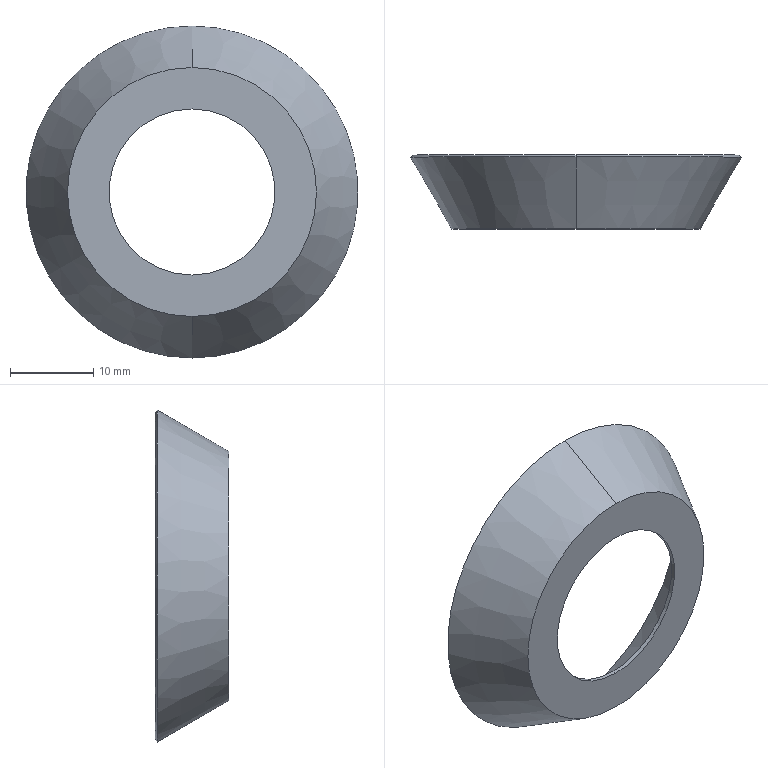Part | SolidWorks | features Revolution 1 | 1 solid | 10 faces | box 40 x 8.91 x 40 mm | volume 725.876 mm3 | cone 6 | cylinder 2 | plane 2 | commonest cylinder face diameters 20 x2
STEP:
#1=CARTESIAN_POINT('',(0.,0.5,-14.711));
#2=VERTEX_POINT('',#1);
#3=CARTESIAN_POINT('',(0.,0.5,14.711));
#4=VERTEX_POINT('',#3);
#5=CARTESIAN_POINT('',(0.,0.5,0.));
#6=DIRECTION('',(0.,1.,0.));
#7=DIRECTION('',(0.,0.,1.));
#8=AXIS2_PLACEMENT_3D('',#5,#6,#7);
#9=CIRCLE('',#8,14.711);
#10=EDGE_CURVE('',#2,#4,#9,.T.);
#11=ORIENTED_EDGE('',*,*,#10,.F.);
#12=CARTESIAN_POINT('',(0.,8.91,-19.567));
#13=VERTEX_POINT('',#12);
#14=CARTESIAN_POINT('',(0.,8.91,-19.567));
#15=DIRECTION('',(0.,0.866,-0.5));
#16=VECTOR('',#15,1000.);
#17=LINE('',#14,#16);
#18=EDGE_CURVE('',#2,#13,#17,.T.);
#19=ORIENTED_EDGE('',*,*,#18,.T.);
#20=CARTESIAN_POINT('',(0.,8.91,19.567));
#21=VERTEX_POINT('',#20);
#22=CARTESIAN_POINT('',(0.,8.91,0.));
#23=DIRECTION('',(0.,1.,0.));
#24=DIRECTION('',(0.,0.,1.));
#25=AXIS2_PLACEMENT_3D('',#22,#23,#24);
#26=CIRCLE('',#25,19.567);
#27=EDGE_CURVE('',#13,#21,#26,.T.);
#28=ORIENTED_EDGE('',*,*,#27,.T.);
#29=CARTESIAN_POINT('',(0.,8.91,19.567));
#30=DIRECTION('',(0.,0.866,0.5));
#31=VECTOR('',#30,1000.);
#32=LINE('',#29,#31);
#33=EDGE_CURVE('',#4,#21,#32,.T.);
#34=ORIENTED_EDGE('',*,*,#33,.F.);
#35=EDGE_LOOP('',(#11,#19,#28,#34));
#36=FACE_OUTER_BOUND('',#35,.T.);
#37=CARTESIAN_POINT('',(0.,8.91,0.));
#38=DIRECTION('',(0.,1.,0.));
#39=DIRECTION('',(0.,0.,1.));
#40=AXIS2_PLACEMENT_3D('',#37,#38,#39);
#41=CONICAL_SURFACE('',#40,19.567,0.5236);
#42=ADVANCED_FACE('',(#36),#41,.F.);
#43=CARTESIAN_POINT('',(0.,8.91,0.));
#44=DIRECTION('',(0.,1.,0.));
#45=DIRECTION('',(0.,0.,1.));
#46=AXIS2_PLACEMENT_3D('',#43,#44,#45);
#47=CIRCLE('',#46,19.567);
#48=EDGE_CURVE('',#21,#13,#47,.T.);
#49=ORIENTED_EDGE('',*,*,#48,.F.);
#50=CARTESIAN_POINT('',(0.,8.66,20.));
#51=VERTEX_POINT('',#50);
#52=CARTESIAN_POINT('',(0.,8.66,20.));
#53=DIRECTION('',(0.,-0.5,0.866));
#54=VECTOR('',#53,1000.);
#55=LINE('',#52,#54);
#56=EDGE_CURVE('',#21,#51,#55,.T.);
#57=ORIENTED_EDGE('',*,*,#56,.T.);
#58=CARTESIAN_POINT('',(0.,8.66,-20.));
#59=VERTEX_POINT('',#58);
#60=CARTESIAN_POINT('',(0.,8.66,0.));
#61=DIRECTION('',(0.,1.,0.));
#62=DIRECTION('',(0.,0.,1.));
#63=AXIS2_PLACEMENT_3D('',#60,#61,#62);
#64=CIRCLE('',#63,20.);
#65=EDGE_CURVE('',#51,#59,#64,.T.);
#66=ORIENTED_EDGE('',*,*,#65,.T.);
#67=CARTESIAN_POINT('',(0.,8.66,-20.));
#68=DIRECTION('',(0.,-0.5,-0.866));
#69=VECTOR('',#68,1000.);
#70=LINE('',#67,#69);
#71=EDGE_CURVE('',#13,#59,#70,.T.);
#72=ORIENTED_EDGE('',*,*,#71,.F.);
#73=EDGE_LOOP('',(#49,#57,#66,#72));
#74=FACE_OUTER_BOUND('',#73,.T.);
#75=CARTESIAN_POINT('',(0.,8.66,0.));
#76=DIRECTION('',(0.,-1.,0.));
#77=DIRECTION('',(0.,0.,-1.));
#78=AXIS2_PLACEMENT_3D('',#75,#76,#77);
#79=CONICAL_SURFACE('',#78,20.,1.047);
#80=ADVANCED_FACE('',(#74),#79,.T.);
#81=CARTESIAN_POINT('',(0.,0.,15.));
#82=VERTEX_POINT('',#81);
#83=CARTESIAN_POINT('',(0.,0.,-15.));
#84=VERTEX_POINT('',#83);
#85=CARTESIAN_POINT('',(0.,0.,0.));
#86=DIRECTION('',(0.,1.,0.));
#87=DIRECTION('',(0.,0.,1.));
#88=AXIS2_PLACEMENT_3D('',#85,#86,#87);
#89=CIRCLE('',#88,15.);
#90=EDGE_CURVE('',#82,#84,#89,.T.);
#91=ORIENTED_EDGE('',*,*,#90,.T.);
#92=CARTESIAN_POINT('',(0.,0.,-15.));
#93=DIRECTION('',(0.,0.866,-0.5));
#94=VECTOR('',#93,1000.);
#95=LINE('',#92,#94);
#96=EDGE_CURVE('',#84,#59,#95,.T.);
#97=ORIENTED_EDGE('',*,*,#96,.T.);
#98=ORIENTED_EDGE('',*,*,#65,.F.);
#99=CARTESIAN_POINT('',(0.,0.,15.));
#100=DIRECTION('',(0.,0.866,0.5));
#101=VECTOR('',#100,1000.);
#102=LINE('',#99,#101);
#103=EDGE_CURVE('',#82,#51,#102,.T.);
#104=ORIENTED_EDGE('',*,*,#103,.F.);
#105=EDGE_LOOP('',(#91,#97,#98,#104));
#106=FACE_OUTER_BOUND('',#105,.T.);
#107=CARTESIAN_POINT('',(0.,0.,0.));
#108=DIRECTION('',(0.,1.,0.));
#109=DIRECTION('',(0.,0.,1.));
#110=AXIS2_PLACEMENT_3D('',#107,#108,#109);
#111=CONICAL_SURFACE('',#110,15.,0.5236);
#112=ADVANCED_FACE('',(#106),#111,.T.);
#113=CARTESIAN_POINT('',(0.,0.,-10.));
#114=VERTEX_POINT('',#113);
#115=CARTESIAN_POINT('',(0.,0.,10.));
#116=VERTEX_POINT('',#115);
#117=CARTESIAN_POINT('',(0.,0.,0.));
#118=DIRECTION('',(0.,1.,0.));
#119=DIRECTION('',(0.,0.,1.));
#120=AXIS2_PLACEMENT_3D('',#117,#118,#119);
#121=CIRCLE('',#120,10.);
#122=EDGE_CURVE('',#114,#116,#121,.T.);
#123=ORIENTED_EDGE('',*,*,#122,.F.);
#124=CARTESIAN_POINT('',(0.,0.5,-10.));
#125=VERTEX_POINT('',#124);
#126=CARTESIAN_POINT('',(0.,20.263,-10.));
#127=DIRECTION('',(0.,1.,0.));
#128=VECTOR('',#127,1000.);
#129=LINE('',#126,#128);
#130=EDGE_CURVE('',#114,#125,#129,.T.);
#131=ORIENTED_EDGE('',*,*,#130,.T.);
#132=CARTESIAN_POINT('',(0.,0.5,10.));
#133=VERTEX_POINT('',#132);
#134=CARTESIAN_POINT('',(0.,0.5,0.));
#135=DIRECTION('',(0.,1.,0.));
#136=DIRECTION('',(0.,0.,1.));
#137=AXIS2_PLACEMENT_3D('',#134,#135,#136);
#138=CIRCLE('',#137,10.);
#139=EDGE_CURVE('',#125,#133,#138,.T.);
#140=ORIENTED_EDGE('',*,*,#139,.T.);
#141=CARTESIAN_POINT('',(0.,20.263,10.));
#142=DIRECTION('',(0.,1.,0.));
#143=VECTOR('',#142,1000.);
#144=LINE('',#141,#143);
#145=EDGE_CURVE('',#116,#133,#144,.T.);
#146=ORIENTED_EDGE('',*,*,#145,.F.);
#147=EDGE_LOOP('',(#123,#131,#140,#146));
#148=FACE_OUTER_BOUND('',#147,.T.);
#149=CARTESIAN_POINT('',(0.,20.263,0.));
#150=DIRECTION('',(0.,1.,0.));
#151=DIRECTION('',(0.,0.,1.));
#152=AXIS2_PLACEMENT_3D('',#149,#150,#151);
#153=CYLINDRICAL_SURFACE('',#152,10.);
#154=ADVANCED_FACE('',(#148),#153,.F.);
#155=ORIENTED_EDGE('',*,*,#130,.F.);
#156=CARTESIAN_POINT('',(0.,0.,0.));
#157=DIRECTION('',(0.,1.,0.));
#158=DIRECTION('',(0.,0.,1.));
#159=AXIS2_PLACEMENT_3D('',#156,#157,#158);
#160=CIRCLE('',#159,10.);
#161=EDGE_CURVE('',#116,#114,#160,.T.);
#162=ORIENTED_EDGE('',*,*,#161,.F.);
#163=ORIENTED_EDGE('',*,*,#145,.T.);
#164=CARTESIAN_POINT('',(0.,0.5,0.));
#165=DIRECTION('',(0.,1.,0.));
#166=DIRECTION('',(0.,0.,1.));
#167=AXIS2_PLACEMENT_3D('',#164,#165,#166);
#168=CIRCLE('',#167,10.);
#169=EDGE_CURVE('',#133,#125,#168,.T.);
#170=ORIENTED_EDGE('',*,*,#169,.T.);
#171=EDGE_LOOP('',(#155,#162,#163,#170));
#172=FACE_OUTER_BOUND('',#171,.T.);
#173=CARTESIAN_POINT('',(0.,20.263,0.));
#174=DIRECTION('',(0.,1.,0.));
#175=DIRECTION('',(0.,0.,1.));
#176=AXIS2_PLACEMENT_3D('',#173,#174,#175);
#177=CYLINDRICAL_SURFACE('',#176,10.);
#178=ADVANCED_FACE('',(#172),#177,.F.);
#179=ORIENTED_EDGE('',*,*,#90,.F.);
#180=CARTESIAN_POINT('',(0.,0.,0.));
#181=DIRECTION('',(0.,1.,0.));
#182=DIRECTION('',(0.,0.,1.));
#183=AXIS2_PLACEMENT_3D('',#180,#181,#182);
#184=CIRCLE('',#183,15.);
#185=EDGE_CURVE('',#84,#82,#184,.T.);
#186=ORIENTED_EDGE('',*,*,#185,.F.);
#187=EDGE_LOOP('',(#179,#186));
#188=FACE_OUTER_BOUND('',#187,.T.);
#189=ORIENTED_EDGE('',*,*,#161,.T.);
#190=ORIENTED_EDGE('',*,*,#122,.T.);
#191=EDGE_LOOP('',(#189,#190));
#192=FACE_BOUND('',#191,.T.);
#193=CARTESIAN_POINT('',(10.,0.,0.));
#194=DIRECTION('',(0.,1.,0.));
#195=DIRECTION('',(0.,0.,1.));
#196=AXIS2_PLACEMENT_3D('',#193,#194,#195);
#197=PLANE('',#196);
#198=ADVANCED_FACE('',(#188,#192),#197,.F.);
#199=ORIENTED_EDGE('',*,*,#96,.F.);
#200=ORIENTED_EDGE('',*,*,#185,.T.);
#201=ORIENTED_EDGE('',*,*,#103,.T.);
#202=CARTESIAN_POINT('',(0.,8.66,0.));
#203=DIRECTION('',(0.,1.,0.));
#204=DIRECTION('',(0.,0.,1.));
#205=AXIS2_PLACEMENT_3D('',#202,#203,#204);
#206=CIRCLE('',#205,20.);
#207=EDGE_CURVE('',#59,#51,#206,.T.);
#208=ORIENTED_EDGE('',*,*,#207,.F.);
#209=EDGE_LOOP('',(#199,#200,#201,#208));
#210=FACE_OUTER_BOUND('',#209,.T.);
#211=CARTESIAN_POINT('',(0.,0.,0.));
#212=DIRECTION('',(0.,1.,0.));
#213=DIRECTION('',(0.,0.,1.));
#214=AXIS2_PLACEMENT_3D('',#211,#212,#213);
#215=CONICAL_SURFACE('',#214,15.,0.5236);
#216=ADVANCED_FACE('',(#210),#215,.T.);
#217=ORIENTED_EDGE('',*,*,#56,.F.);
#218=ORIENTED_EDGE('',*,*,#27,.F.);
#219=ORIENTED_EDGE('',*,*,#71,.T.);
#220=ORIENTED_EDGE('',*,*,#207,.T.);
#221=EDGE_LOOP('',(#217,#218,#219,#220));
#222=FACE_OUTER_BOUND('',#221,.T.);
#223=CARTESIAN_POINT('',(0.,8.66,0.));
#224=DIRECTION('',(0.,-1.,0.));
#225=DIRECTION('',(0.,0.,-1.));
#226=AXIS2_PLACEMENT_3D('',#223,#224,#225);
#227=CONICAL_SURFACE('',#226,20.,1.047);
#228=ADVANCED_FACE('',(#222),#227,.T.);
#229=ORIENTED_EDGE('',*,*,#18,.F.);
#230=CARTESIAN_POINT('',(0.,0.5,0.));
#231=DIRECTION('',(0.,1.,0.));
#232=DIRECTION('',(0.,0.,1.));
#233=AXIS2_PLACEMENT_3D('',#230,#231,#232);
#234=CIRCLE('',#233,14.711);
#235=EDGE_CURVE('',#4,#2,#234,.T.);
#236=ORIENTED_EDGE('',*,*,#235,.F.);
#237=ORIENTED_EDGE('',*,*,#33,.T.);
#238=ORIENTED_EDGE('',*,*,#48,.T.);
#239=EDGE_LOOP('',(#229,#236,#237,#238));
#240=FACE_OUTER_BOUND('',#239,.T.);
#241=CARTESIAN_POINT('',(0.,8.91,0.));
#242=DIRECTION('',(0.,1.,0.));
#243=DIRECTION('',(0.,0.,1.));
#244=AXIS2_PLACEMENT_3D('',#241,#242,#243);
#245=CONICAL_SURFACE('',#244,19.567,0.5236);
#246=ADVANCED_FACE('',(#240),#245,.F.);
#247=ORIENTED_EDGE('',*,*,#169,.F.);
#248=ORIENTED_EDGE('',*,*,#139,.F.);
#249=EDGE_LOOP('',(#247,#248));
#250=FACE_BOUND('',#249,.T.);
#251=ORIENTED_EDGE('',*,*,#235,.T.);
#252=ORIENTED_EDGE('',*,*,#10,.T.);
#253=EDGE_LOOP('',(#251,#252));
#254=FACE_OUTER_BOUND('',#253,.T.);
#255=CARTESIAN_POINT('',(10.,0.5,0.));
#256=DIRECTION('',(0.,-1.,0.));
#257=DIRECTION('',(0.,0.,-1.));
#258=AXIS2_PLACEMENT_3D('',#255,#256,#257);
#259=PLANE('',#258);
#260=ADVANCED_FACE('',(#250,#254),#259,.F.);
#261=CLOSED_SHELL('',(#42,#80,#112,#154,#178,#198,#216,#228,#246,#260));
#262=MANIFOLD_SOLID_BREP('',#261);
#263=CARTESIAN_POINT('',(0.,0.,0.));
#264=DIRECTION('',(0.,0.,1.));
#265=DIRECTION('',(1.,0.,0.));
#266=AXIS2_PLACEMENT_3D('',#263,#264,#265);
#267=(LENGTH_UNIT()NAMED_UNIT(*)SI_UNIT(.MILLI.,.METRE.));
#268=UNCERTAINTY_MEASURE_WITH_UNIT(LENGTH_MEASURE(0.00001),#267,'','');
#269=(NAMED_UNIT(*)PLANE_ANGLE_UNIT()SI_UNIT($,.RADIAN.));
#270=(NAMED_UNIT(*)SI_UNIT($,.STERADIAN.)SOLID_ANGLE_UNIT());
#271=(GEOMETRIC_REPRESENTATION_CONTEXT(3)GLOBAL_UNCERTAINTY_ASSIGNED_CONTEXT((#268))GLOBAL_UNIT_ASSIGNED_CONTEXT((#267,#269,#270))REPRESENTATION_CONTEXT('',''));
#272=ADVANCED_BREP_SHAPE_REPRESENTATION('',(#262,#266),#271);